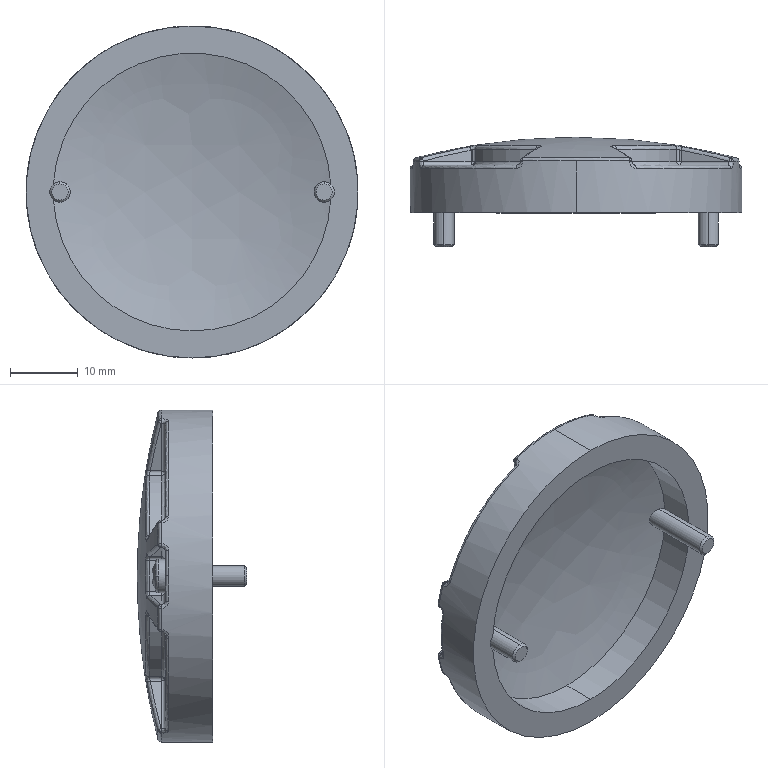Part | STEP file | FCG-80 | 1 solid | 253 faces | box 49 x 16.126 x 49 mm | volume 8270 mm3 | spline 121 | plane 69 | cylinder 59 | cone 4 | commonest cylinder face diameters 1 x40 32 x6 3 x4 5 x4 41 x3 49 x2